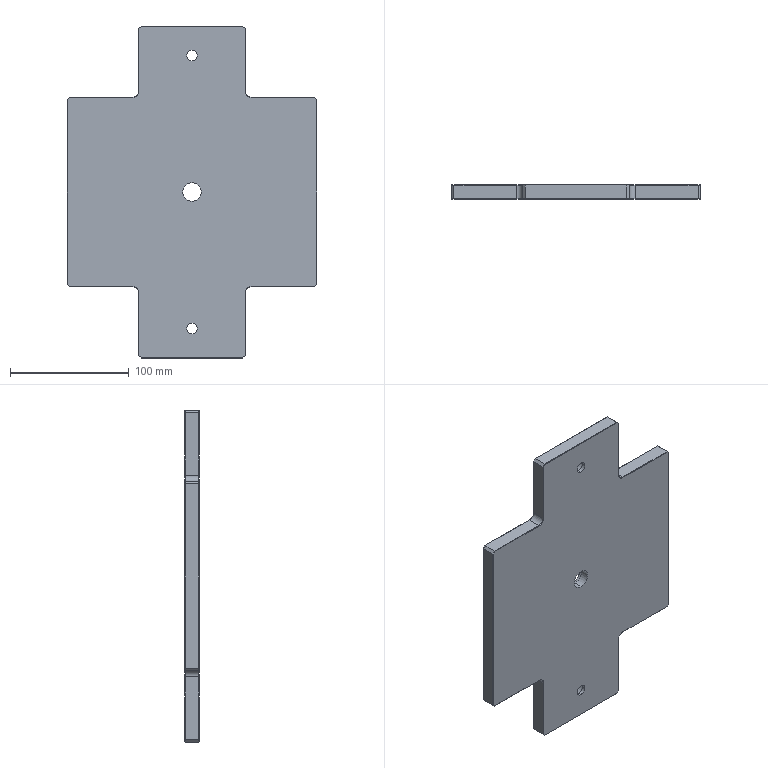Part | SolidWorks | features ICE 4, Chamfer 3, Extrusion 1, Fillet 1 | 1 solid | 89 faces | box 210 x 12 x 280 mm | volume 525634 mm3 | plane 65 | cylinder 16 | cone 8 | commonest cylinder face diameters 9 x4 10 x4 15 x4 15.5 x2 24 x2